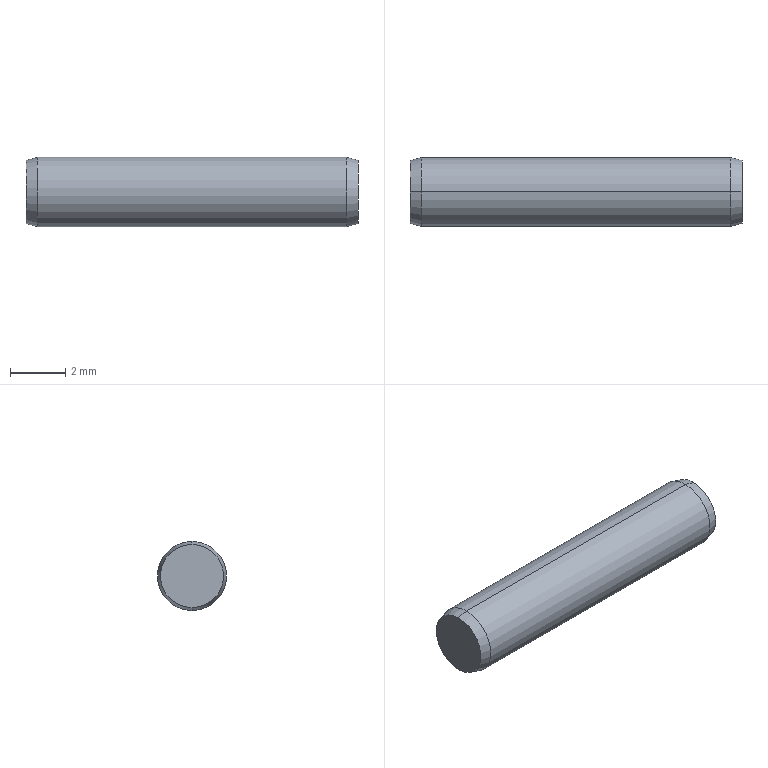Part | SolidWorks | features Revolution 1 | 1 solid | 8 faces | box 12 x 2.5 x 2.5 mm | volume 58.578 mm3 | cone 4 | cylinder 2 | plane 2 | commonest cylinder face diameters 2.5 x2
STEP:
#1=CARTESIAN_POINT('',(10.2,0.,1.25));
#2=VERTEX_POINT('',#1);
#3=CARTESIAN_POINT('',(10.2,0.,-1.25));
#4=VERTEX_POINT('',#3);
#5=CARTESIAN_POINT('',(10.2,0.,0.));
#6=DIRECTION('',(-1.,0.,0.));
#7=DIRECTION('',(0.,0.,1.));
#8=AXIS2_PLACEMENT_3D('',#5,#6,#7);
#9=CIRCLE('',#8,1.25);
#10=EDGE_CURVE('',#2,#4,#9,.T.);
#11=ORIENTED_EDGE('',*,*,#10,.T.);
#12=CARTESIAN_POINT('',(-1.,0.,-1.25));
#13=VERTEX_POINT('',#12);
#14=CARTESIAN_POINT('',(0.,0.,-1.25));
#15=DIRECTION('',(-1.,0.,0.));
#16=VECTOR('',#15,1000.);
#17=LINE('',#14,#16);
#18=EDGE_CURVE('',#4,#13,#17,.T.);
#19=ORIENTED_EDGE('',*,*,#18,.T.);
#20=CARTESIAN_POINT('',(-1.,0.,1.25));
#21=VERTEX_POINT('',#20);
#22=CARTESIAN_POINT('',(-1.,0.,0.));
#23=DIRECTION('',(-1.,0.,0.));
#24=DIRECTION('',(0.,0.,1.));
#25=AXIS2_PLACEMENT_3D('',#22,#23,#24);
#26=CIRCLE('',#25,1.25);
#27=EDGE_CURVE('',#21,#13,#26,.T.);
#28=ORIENTED_EDGE('',*,*,#27,.F.);
#29=CARTESIAN_POINT('',(0.,0.,1.25));
#30=DIRECTION('',(-1.,0.,0.));
#31=VECTOR('',#30,1000.);
#32=LINE('',#29,#31);
#33=EDGE_CURVE('',#2,#21,#32,.T.);
#34=ORIENTED_EDGE('',*,*,#33,.F.);
#35=EDGE_LOOP('',(#11,#19,#28,#34));
#36=FACE_OUTER_BOUND('',#35,.T.);
#37=CARTESIAN_POINT('',(0.,0.,0.));
#38=DIRECTION('',(-1.,0.,0.));
#39=DIRECTION('',(0.,0.,1.));
#40=AXIS2_PLACEMENT_3D('',#37,#38,#39);
#41=CYLINDRICAL_SURFACE('',#40,1.25);
#42=ADVANCED_FACE('',(#36),#41,.T.);
#43=CARTESIAN_POINT('',(-1.4,0.,1.143));
#44=VERTEX_POINT('',#43);
#45=CARTESIAN_POINT('',(-1.4,0.,-1.143));
#46=VERTEX_POINT('',#45);
#47=CARTESIAN_POINT('',(-1.4,0.,0.));
#48=DIRECTION('',(-1.,0.,0.));
#49=DIRECTION('',(0.,0.,1.));
#50=AXIS2_PLACEMENT_3D('',#47,#48,#49);
#51=CIRCLE('',#50,1.143);
#52=EDGE_CURVE('',#44,#46,#51,.T.);
#53=ORIENTED_EDGE('',*,*,#52,.F.);
#54=CARTESIAN_POINT('',(-1.,0.,1.25));
#55=DIRECTION('',(0.9659,0.,0.2588));
#56=VECTOR('',#55,1000.);
#57=LINE('',#54,#56);
#58=EDGE_CURVE('',#44,#21,#57,.T.);
#59=ORIENTED_EDGE('',*,*,#58,.T.);
#60=ORIENTED_EDGE('',*,*,#27,.T.);
#61=CARTESIAN_POINT('',(-1.,0.,-1.25));
#62=DIRECTION('',(0.9659,0.,-0.2588));
#63=VECTOR('',#62,1000.);
#64=LINE('',#61,#63);
#65=EDGE_CURVE('',#46,#13,#64,.T.);
#66=ORIENTED_EDGE('',*,*,#65,.F.);
#67=EDGE_LOOP('',(#53,#59,#60,#66));
#68=FACE_OUTER_BOUND('',#67,.T.);
#69=CARTESIAN_POINT('',(-1.,0.,0.));
#70=DIRECTION('',(1.,0.,0.));
#71=DIRECTION('',(0.,0.,-1.));
#72=AXIS2_PLACEMENT_3D('',#69,#70,#71);
#73=CONICAL_SURFACE('',#72,1.25,0.2618);
#74=ADVANCED_FACE('',(#68),#73,.T.);
#75=CARTESIAN_POINT('',(10.6,0.,1.143));
#76=VERTEX_POINT('',#75);
#77=CARTESIAN_POINT('',(10.6,0.,-1.143));
#78=VERTEX_POINT('',#77);
#79=CARTESIAN_POINT('',(10.6,0.,0.));
#80=DIRECTION('',(-1.,0.,0.));
#81=DIRECTION('',(0.,0.,1.));
#82=AXIS2_PLACEMENT_3D('',#79,#80,#81);
#83=CIRCLE('',#82,1.143);
#84=EDGE_CURVE('',#76,#78,#83,.T.);
#85=ORIENTED_EDGE('',*,*,#84,.T.);
#86=CARTESIAN_POINT('',(10.6,0.,-1.143));
#87=DIRECTION('',(-0.9659,0.,-0.2588));
#88=VECTOR('',#87,1000.);
#89=LINE('',#86,#88);
#90=EDGE_CURVE('',#78,#4,#89,.T.);
#91=ORIENTED_EDGE('',*,*,#90,.T.);
#92=ORIENTED_EDGE('',*,*,#10,.F.);
#93=CARTESIAN_POINT('',(10.6,0.,1.143));
#94=DIRECTION('',(-0.9659,0.,0.2588));
#95=VECTOR('',#94,1000.);
#96=LINE('',#93,#95);
#97=EDGE_CURVE('',#76,#2,#96,.T.);
#98=ORIENTED_EDGE('',*,*,#97,.F.);
#99=EDGE_LOOP('',(#85,#91,#92,#98));
#100=FACE_OUTER_BOUND('',#99,.T.);
#101=CARTESIAN_POINT('',(10.6,0.,0.));
#102=DIRECTION('',(-1.,0.,0.));
#103=DIRECTION('',(0.,0.,1.));
#104=AXIS2_PLACEMENT_3D('',#101,#102,#103);
#105=CONICAL_SURFACE('',#104,1.143,0.2618);
#106=ADVANCED_FACE('',(#100),#105,.T.);
#107=ORIENTED_EDGE('',*,*,#90,.F.);
#108=CARTESIAN_POINT('',(10.6,0.,0.));
#109=DIRECTION('',(-1.,0.,0.));
#110=DIRECTION('',(0.,0.,1.));
#111=AXIS2_PLACEMENT_3D('',#108,#109,#110);
#112=CIRCLE('',#111,1.143);
#113=EDGE_CURVE('',#78,#76,#112,.T.);
#114=ORIENTED_EDGE('',*,*,#113,.T.);
#115=ORIENTED_EDGE('',*,*,#97,.T.);
#116=CARTESIAN_POINT('',(10.2,0.,0.));
#117=DIRECTION('',(-1.,0.,0.));
#118=DIRECTION('',(0.,0.,1.));
#119=AXIS2_PLACEMENT_3D('',#116,#117,#118);
#120=CIRCLE('',#119,1.25);
#121=EDGE_CURVE('',#4,#2,#120,.T.);
#122=ORIENTED_EDGE('',*,*,#121,.F.);
#123=EDGE_LOOP('',(#107,#114,#115,#122));
#124=FACE_OUTER_BOUND('',#123,.T.);
#125=CARTESIAN_POINT('',(10.6,0.,0.));
#126=DIRECTION('',(-1.,0.,0.));
#127=DIRECTION('',(0.,0.,1.));
#128=AXIS2_PLACEMENT_3D('',#125,#126,#127);
#129=CONICAL_SURFACE('',#128,1.143,0.2618);
#130=ADVANCED_FACE('',(#124),#129,.T.);
#131=ORIENTED_EDGE('',*,*,#84,.F.);
#132=ORIENTED_EDGE('',*,*,#113,.F.);
#133=EDGE_LOOP('',(#131,#132));
#134=FACE_OUTER_BOUND('',#133,.T.);
#135=CARTESIAN_POINT('',(10.6,1.143,0.));
#136=DIRECTION('',(-1.,0.,0.));
#137=DIRECTION('',(0.,0.,1.));
#138=AXIS2_PLACEMENT_3D('',#135,#136,#137);
#139=PLANE('',#138);
#140=ADVANCED_FACE('',(#134),#139,.F.);
#141=CARTESIAN_POINT('',(-1.4,0.,0.));
#142=DIRECTION('',(-1.,0.,0.));
#143=DIRECTION('',(0.,0.,1.));
#144=AXIS2_PLACEMENT_3D('',#141,#142,#143);
#145=CIRCLE('',#144,1.143);
#146=EDGE_CURVE('',#46,#44,#145,.T.);
#147=ORIENTED_EDGE('',*,*,#146,.T.);
#148=ORIENTED_EDGE('',*,*,#52,.T.);
#149=EDGE_LOOP('',(#147,#148));
#150=FACE_OUTER_BOUND('',#149,.T.);
#151=CARTESIAN_POINT('',(-1.4,1.143,0.));
#152=DIRECTION('',(1.,0.,0.));
#153=DIRECTION('',(0.,0.,-1.));
#154=AXIS2_PLACEMENT_3D('',#151,#152,#153);
#155=PLANE('',#154);
#156=ADVANCED_FACE('',(#150),#155,.F.);
#157=ORIENTED_EDGE('',*,*,#58,.F.);
#158=ORIENTED_EDGE('',*,*,#146,.F.);
#159=ORIENTED_EDGE('',*,*,#65,.T.);
#160=CARTESIAN_POINT('',(-1.,0.,0.));
#161=DIRECTION('',(-1.,0.,0.));
#162=DIRECTION('',(0.,0.,1.));
#163=AXIS2_PLACEMENT_3D('',#160,#161,#162);
#164=CIRCLE('',#163,1.25);
#165=EDGE_CURVE('',#13,#21,#164,.T.);
#166=ORIENTED_EDGE('',*,*,#165,.T.);
#167=EDGE_LOOP('',(#157,#158,#159,#166));
#168=FACE_OUTER_BOUND('',#167,.T.);
#169=CARTESIAN_POINT('',(-1.,0.,0.));
#170=DIRECTION('',(1.,0.,0.));
#171=DIRECTION('',(0.,0.,-1.));
#172=AXIS2_PLACEMENT_3D('',#169,#170,#171);
#173=CONICAL_SURFACE('',#172,1.25,0.2618);
#174=ADVANCED_FACE('',(#168),#173,.T.);
#175=ORIENTED_EDGE('',*,*,#18,.F.);
#176=ORIENTED_EDGE('',*,*,#121,.T.);
#177=ORIENTED_EDGE('',*,*,#33,.T.);
#178=ORIENTED_EDGE('',*,*,#165,.F.);
#179=EDGE_LOOP('',(#175,#176,#177,#178));
#180=FACE_OUTER_BOUND('',#179,.T.);
#181=CARTESIAN_POINT('',(0.,0.,0.));
#182=DIRECTION('',(-1.,0.,0.));
#183=DIRECTION('',(0.,0.,1.));
#184=AXIS2_PLACEMENT_3D('',#181,#182,#183);
#185=CYLINDRICAL_SURFACE('',#184,1.25);
#186=ADVANCED_FACE('',(#180),#185,.T.);
#187=CLOSED_SHELL('',(#42,#74,#106,#130,#140,#156,#174,#186));
#188=MANIFOLD_SOLID_BREP('',#187);
#189=CARTESIAN_POINT('',(0.,0.,0.));
#190=DIRECTION('',(0.,0.,1.));
#191=DIRECTION('',(1.,0.,0.));
#192=AXIS2_PLACEMENT_3D('',#189,#190,#191);
#193=(LENGTH_UNIT()NAMED_UNIT(*)SI_UNIT(.MILLI.,.METRE.));
#194=UNCERTAINTY_MEASURE_WITH_UNIT(LENGTH_MEASURE(0.00001),#193,'','');
#195=(NAMED_UNIT(*)PLANE_ANGLE_UNIT()SI_UNIT($,.RADIAN.));
#196=(NAMED_UNIT(*)SI_UNIT($,.STERADIAN.)SOLID_ANGLE_UNIT());
#197=(GEOMETRIC_REPRESENTATION_CONTEXT(3)GLOBAL_UNCERTAINTY_ASSIGNED_CONTEXT((#194))GLOBAL_UNIT_ASSIGNED_CONTEXT((#193,#195,#196))REPRESENTATION_CONTEXT('',''));
#198=ADVANCED_BREP_SHAPE_REPRESENTATION('',(#188,#192),#197);